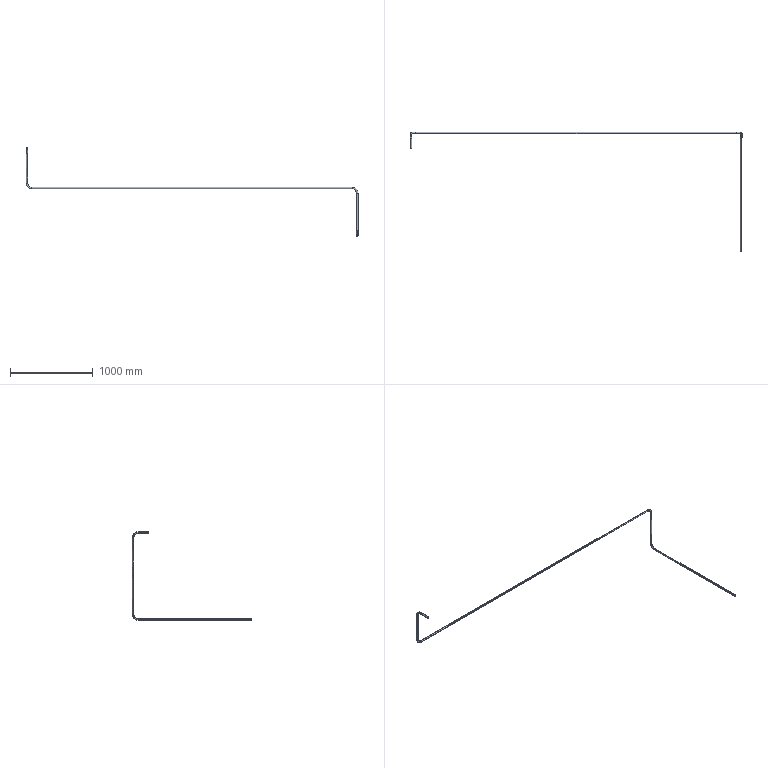Part | SolidWorks | features 3DProfileFeature 2, Sweep 1 | 1 solid | 38 faces | box 4020 x 1445 x 1070 mm | volume 1547370 mm3 | cylinder 20 | torus 16 | plane 2 | commonest cylinder face diameters 10 x10 20 x10
STEP:
#1=CARTESIAN_POINT('',(-1700.,3089.387,-104.234));
#2=VERTEX_POINT('',#1);
#3=CARTESIAN_POINT('',(-1705.,3084.387,-104.234));
#4=VERTEX_POINT('',#3);
#5=CARTESIAN_POINT('',(-1700.,3084.387,-104.234));
#6=DIRECTION('',(0.,0.,1.));
#7=DIRECTION('',(-1.,0.,0.));
#8=AXIS2_PLACEMENT_3D('',#5,#6,#7);
#9=CIRCLE('',#8,5.);
#10=EDGE_CURVE('',#2,#4,#9,.T.);
#11=ORIENTED_EDGE('',*,*,#10,.F.);
#12=CARTESIAN_POINT('',(-1700.,3024.387,-39.234));
#13=VERTEX_POINT('',#12);
#14=CARTESIAN_POINT('',(-1700.,3024.387,-104.234));
#15=DIRECTION('',(1.,0.,0.));
#16=DIRECTION('',(0.,0.,-1.));
#17=AXIS2_PLACEMENT_3D('',#14,#15,#16);
#18=CIRCLE('',#17,65.);
#19=EDGE_CURVE('',#2,#13,#18,.T.);
#20=ORIENTED_EDGE('',*,*,#19,.T.);
#21=CARTESIAN_POINT('',(-1700.,3024.387,-49.234));
#22=VERTEX_POINT('',#21);
#23=CARTESIAN_POINT('',(-1700.,3024.387,-44.234));
#24=DIRECTION('',(0.,-1.,0.));
#25=DIRECTION('',(0.,0.,-1.));
#26=AXIS2_PLACEMENT_3D('',#23,#24,#25);
#27=CIRCLE('',#26,5.);
#28=EDGE_CURVE('',#13,#22,#27,.T.);
#29=ORIENTED_EDGE('',*,*,#28,.T.);
#30=CARTESIAN_POINT('',(-1700.,3079.387,-104.234));
#31=VERTEX_POINT('',#30);
#32=CARTESIAN_POINT('',(-1700.,3024.387,-104.234));
#33=DIRECTION('',(1.,0.,0.));
#34=DIRECTION('',(0.,0.,-1.));
#35=AXIS2_PLACEMENT_3D('',#32,#33,#34);
#36=CIRCLE('',#35,55.);
#37=EDGE_CURVE('',#31,#22,#36,.T.);
#38=ORIENTED_EDGE('',*,*,#37,.F.);
#39=CARTESIAN_POINT('',(-1700.,3084.387,-104.234));
#40=DIRECTION('',(0.,0.,1.));
#41=DIRECTION('',(-1.,0.,0.));
#42=AXIS2_PLACEMENT_3D('',#39,#40,#41);
#43=CIRCLE('',#42,5.);
#44=EDGE_CURVE('',#4,#31,#43,.T.);
#45=ORIENTED_EDGE('',*,*,#44,.F.);
#46=EDGE_LOOP('',(#11,#20,#29,#38,#45));
#47=FACE_OUTER_BOUND('',#46,.T.);
#48=CARTESIAN_POINT('',(-1700.,3024.387,-104.234));
#49=DIRECTION('',(1.,0.,0.));
#50=DIRECTION('',(0.,0.,-1.));
#51=AXIS2_PLACEMENT_3D('',#48,#49,#50);
#52=TOROIDAL_SURFACE('',#51,60.,5.);
#53=ADVANCED_FACE('',(#47),#52,.F.);
#54=CARTESIAN_POINT('',(-1640.,3084.387,-526.487));
#55=VERTEX_POINT('',#54);
#56=CARTESIAN_POINT('',(-1640.,3084.387,-516.487));
#57=VERTEX_POINT('',#56);
#58=CARTESIAN_POINT('',(-1640.,3084.387,-521.487));
#59=DIRECTION('',(-1.,0.,0.));
#60=DIRECTION('',(0.,0.,-1.));
#61=AXIS2_PLACEMENT_3D('',#58,#59,#60);
#62=CIRCLE('',#61,5.);
#63=EDGE_CURVE('',#55,#57,#62,.T.);
#64=ORIENTED_EDGE('',*,*,#63,.F.);
#65=CARTESIAN_POINT('',(-1705.,3084.387,-461.487));
#66=VERTEX_POINT('',#65);
#67=CARTESIAN_POINT('',(-1640.,3084.387,-461.487));
#68=DIRECTION('',(0.,1.,0.));
#69=DIRECTION('',(0.,0.,1.));
#70=AXIS2_PLACEMENT_3D('',#67,#68,#69);
#71=CIRCLE('',#70,65.);
#72=EDGE_CURVE('',#55,#66,#71,.T.);
#73=ORIENTED_EDGE('',*,*,#72,.T.);
#74=CARTESIAN_POINT('',(-1695.,3084.387,-461.487));
#75=VERTEX_POINT('',#74);
#76=CARTESIAN_POINT('',(-1700.,3084.387,-461.487));
#77=DIRECTION('',(0.,0.,1.));
#78=DIRECTION('',(1.,0.,0.));
#79=AXIS2_PLACEMENT_3D('',#76,#77,#78);
#80=CIRCLE('',#79,5.);
#81=EDGE_CURVE('',#66,#75,#80,.T.);
#82=ORIENTED_EDGE('',*,*,#81,.T.);
#83=CARTESIAN_POINT('',(-1640.,3084.387,-461.487));
#84=DIRECTION('',(0.,1.,0.));
#85=DIRECTION('',(0.,0.,1.));
#86=AXIS2_PLACEMENT_3D('',#83,#84,#85);
#87=CIRCLE('',#86,55.);
#88=EDGE_CURVE('',#57,#75,#87,.T.);
#89=ORIENTED_EDGE('',*,*,#88,.F.);
#90=EDGE_LOOP('',(#64,#73,#82,#89));
#91=FACE_OUTER_BOUND('',#90,.T.);
#92=CARTESIAN_POINT('',(-1640.,3084.387,-461.487));
#93=DIRECTION('',(0.,1.,0.));
#94=DIRECTION('',(0.,0.,1.));
#95=AXIS2_PLACEMENT_3D('',#92,#93,#94);
#96=TOROIDAL_SURFACE('',#95,60.,5.);
#97=ADVANCED_FACE('',(#91),#96,.F.);
#98=CARTESIAN_POINT('',(2305.,3084.387,-581.487));
#99=VERTEX_POINT('',#98);
#100=CARTESIAN_POINT('',(2295.,3084.387,-581.487));
#101=VERTEX_POINT('',#100);
#102=CARTESIAN_POINT('',(2300.,3084.387,-581.487));
#103=DIRECTION('',(0.,0.,1.));
#104=DIRECTION('',(-1.,0.,0.));
#105=AXIS2_PLACEMENT_3D('',#102,#103,#104);
#106=CIRCLE('',#105,5.);
#107=EDGE_CURVE('',#99,#101,#106,.T.);
#108=ORIENTED_EDGE('',*,*,#107,.F.);
#109=CARTESIAN_POINT('',(2240.,3084.387,-516.487));
#110=VERTEX_POINT('',#109);
#111=CARTESIAN_POINT('',(2240.,3084.387,-581.487));
#112=DIRECTION('',(0.,-1.,0.));
#113=DIRECTION('',(0.,0.,-1.));
#114=AXIS2_PLACEMENT_3D('',#111,#112,#113);
#115=CIRCLE('',#114,65.);
#116=EDGE_CURVE('',#99,#110,#115,.T.);
#117=ORIENTED_EDGE('',*,*,#116,.T.);
#118=CARTESIAN_POINT('',(2240.,3084.387,-526.487));
#119=VERTEX_POINT('',#118);
#120=CARTESIAN_POINT('',(2240.,3084.387,-521.487));
#121=DIRECTION('',(-1.,0.,0.));
#122=DIRECTION('',(0.,0.,1.));
#123=AXIS2_PLACEMENT_3D('',#120,#121,#122);
#124=CIRCLE('',#123,5.);
#125=EDGE_CURVE('',#110,#119,#124,.T.);
#126=ORIENTED_EDGE('',*,*,#125,.T.);
#127=CARTESIAN_POINT('',(2240.,3084.387,-581.487));
#128=DIRECTION('',(0.,-1.,0.));
#129=DIRECTION('',(0.,0.,-1.));
#130=AXIS2_PLACEMENT_3D('',#127,#128,#129);
#131=CIRCLE('',#130,55.);
#132=EDGE_CURVE('',#101,#119,#131,.T.);
#133=ORIENTED_EDGE('',*,*,#132,.F.);
#134=EDGE_LOOP('',(#108,#117,#126,#133));
#135=FACE_OUTER_BOUND('',#134,.T.);
#136=CARTESIAN_POINT('',(2240.,3084.387,-581.487));
#137=DIRECTION('',(0.,-1.,0.));
#138=DIRECTION('',(0.,0.,-1.));
#139=AXIS2_PLACEMENT_3D('',#136,#137,#138);
#140=TOROIDAL_SURFACE('',#139,60.,5.);
#141=ADVANCED_FACE('',(#135),#140,.F.);
#142=CARTESIAN_POINT('',(2300.,3024.387,-1099.234));
#143=VERTEX_POINT('',#142);
#144=CARTESIAN_POINT('',(2300.,3024.387,-1089.234));
#145=VERTEX_POINT('',#144);
#146=CARTESIAN_POINT('',(2300.,3024.387,-1094.234));
#147=DIRECTION('',(0.,1.,0.));
#148=DIRECTION('',(0.,0.,-1.));
#149=AXIS2_PLACEMENT_3D('',#146,#147,#148);
#150=CIRCLE('',#149,5.);
#151=EDGE_CURVE('',#143,#145,#150,.T.);
#152=ORIENTED_EDGE('',*,*,#151,.F.);
#153=CARTESIAN_POINT('',(2300.,3089.387,-1034.234));
#154=VERTEX_POINT('',#153);
#155=CARTESIAN_POINT('',(2300.,3024.387,-1034.234));
#156=DIRECTION('',(1.,0.,0.));
#157=DIRECTION('',(0.,0.,-1.));
#158=AXIS2_PLACEMENT_3D('',#155,#156,#157);
#159=CIRCLE('',#158,65.);
#160=EDGE_CURVE('',#143,#154,#159,.T.);
#161=ORIENTED_EDGE('',*,*,#160,.T.);
#162=CARTESIAN_POINT('',(2295.,3084.387,-1034.234));
#163=VERTEX_POINT('',#162);
#164=CARTESIAN_POINT('',(2300.,3084.387,-1034.234));
#165=DIRECTION('',(0.,0.,1.));
#166=DIRECTION('',(1.,0.,0.));
#167=AXIS2_PLACEMENT_3D('',#164,#165,#166);
#168=CIRCLE('',#167,5.);
#169=EDGE_CURVE('',#154,#163,#168,.T.);
#170=ORIENTED_EDGE('',*,*,#169,.T.);
#171=CARTESIAN_POINT('',(2300.,3079.387,-1034.234));
#172=VERTEX_POINT('',#171);
#173=CARTESIAN_POINT('',(2300.,3084.387,-1034.234));
#174=DIRECTION('',(0.,0.,1.));
#175=DIRECTION('',(1.,0.,0.));
#176=AXIS2_PLACEMENT_3D('',#173,#174,#175);
#177=CIRCLE('',#176,5.);
#178=EDGE_CURVE('',#163,#172,#177,.T.);
#179=ORIENTED_EDGE('',*,*,#178,.T.);
#180=CARTESIAN_POINT('',(2300.,3024.387,-1034.234));
#181=DIRECTION('',(1.,0.,0.));
#182=DIRECTION('',(0.,0.,-1.));
#183=AXIS2_PLACEMENT_3D('',#180,#181,#182);
#184=CIRCLE('',#183,55.);
#185=EDGE_CURVE('',#145,#172,#184,.T.);
#186=ORIENTED_EDGE('',*,*,#185,.F.);
#187=EDGE_LOOP('',(#152,#161,#170,#179,#186));
#188=FACE_OUTER_BOUND('',#187,.T.);
#189=CARTESIAN_POINT('',(2300.,3024.387,-1034.234));
#190=DIRECTION('',(1.,0.,0.));
#191=DIRECTION('',(0.,0.,-1.));
#192=AXIS2_PLACEMENT_3D('',#189,#190,#191);
#193=TOROIDAL_SURFACE('',#192,60.,5.);
#194=ADVANCED_FACE('',(#188),#193,.F.);
#195=CARTESIAN_POINT('',(-1690.,3084.387,-104.234));
#196=VERTEX_POINT('',#195);
#197=CARTESIAN_POINT('',(-1700.,3094.387,-104.234));
#198=VERTEX_POINT('',#197);
#199=CARTESIAN_POINT('',(-1700.,3084.387,-104.234));
#200=DIRECTION('',(0.,0.,1.));
#201=DIRECTION('',(0.,-1.,0.));
#202=AXIS2_PLACEMENT_3D('',#199,#200,#201);
#203=CIRCLE('',#202,10.);
#204=EDGE_CURVE('',#196,#198,#203,.T.);
#205=ORIENTED_EDGE('',*,*,#204,.T.);
#206=CARTESIAN_POINT('',(-1700.,3024.387,-34.234));
#207=VERTEX_POINT('',#206);
#208=CARTESIAN_POINT('',(-1700.,3024.387,-104.234));
#209=DIRECTION('',(1.,0.,0.));
#210=DIRECTION('',(0.,0.,-1.));
#211=AXIS2_PLACEMENT_3D('',#208,#209,#210);
#212=CIRCLE('',#211,70.);
#213=EDGE_CURVE('',#198,#207,#212,.T.);
#214=ORIENTED_EDGE('',*,*,#213,.T.);
#215=CARTESIAN_POINT('',(-1700.,3024.387,-54.234));
#216=VERTEX_POINT('',#215);
#217=CARTESIAN_POINT('',(-1700.,3024.387,-44.234));
#218=DIRECTION('',(0.,-1.,0.));
#219=DIRECTION('',(0.,0.,-1.));
#220=AXIS2_PLACEMENT_3D('',#217,#218,#219);
#221=CIRCLE('',#220,10.);
#222=EDGE_CURVE('',#216,#207,#221,.T.);
#223=ORIENTED_EDGE('',*,*,#222,.F.);
#224=CARTESIAN_POINT('',(-1700.,3074.387,-104.234));
#225=VERTEX_POINT('',#224);
#226=CARTESIAN_POINT('',(-1700.,3024.387,-104.234));
#227=DIRECTION('',(1.,0.,0.));
#228=DIRECTION('',(0.,0.,-1.));
#229=AXIS2_PLACEMENT_3D('',#226,#227,#228);
#230=CIRCLE('',#229,50.);
#231=EDGE_CURVE('',#225,#216,#230,.T.);
#232=ORIENTED_EDGE('',*,*,#231,.F.);
#233=CARTESIAN_POINT('',(-1700.,3084.387,-104.234));
#234=DIRECTION('',(0.,0.,1.));
#235=DIRECTION('',(0.,-1.,0.));
#236=AXIS2_PLACEMENT_3D('',#233,#234,#235);
#237=CIRCLE('',#236,10.);
#238=EDGE_CURVE('',#225,#196,#237,.T.);
#239=ORIENTED_EDGE('',*,*,#238,.T.);
#240=EDGE_LOOP('',(#205,#214,#223,#232,#239));
#241=FACE_OUTER_BOUND('',#240,.T.);
#242=CARTESIAN_POINT('',(-1700.,3024.387,-104.234));
#243=DIRECTION('',(1.,0.,0.));
#244=DIRECTION('',(0.,0.,-1.));
#245=AXIS2_PLACEMENT_3D('',#242,#243,#244);
#246=TOROIDAL_SURFACE('',#245,60.,10.);
#247=ADVANCED_FACE('',(#241),#246,.T.);
#248=CARTESIAN_POINT('',(-1640.,3084.387,-511.487));
#249=VERTEX_POINT('',#248);
#250=CARTESIAN_POINT('',(-1640.,3084.387,-531.487));
#251=VERTEX_POINT('',#250);
#252=CARTESIAN_POINT('',(-1640.,3084.387,-521.487));
#253=DIRECTION('',(-1.,0.,0.));
#254=DIRECTION('',(0.,-1.,0.));
#255=AXIS2_PLACEMENT_3D('',#252,#253,#254);
#256=CIRCLE('',#255,10.);
#257=EDGE_CURVE('',#249,#251,#256,.T.);
#258=ORIENTED_EDGE('',*,*,#257,.T.);
#259=CARTESIAN_POINT('',(-1710.,3084.387,-461.487));
#260=VERTEX_POINT('',#259);
#261=CARTESIAN_POINT('',(-1640.,3084.387,-461.487));
#262=DIRECTION('',(0.,1.,0.));
#263=DIRECTION('',(0.,0.,1.));
#264=AXIS2_PLACEMENT_3D('',#261,#262,#263);
#265=CIRCLE('',#264,70.);
#266=EDGE_CURVE('',#251,#260,#265,.T.);
#267=ORIENTED_EDGE('',*,*,#266,.T.);
#268=CARTESIAN_POINT('',(-1690.,3084.387,-461.487));
#269=VERTEX_POINT('',#268);
#270=CARTESIAN_POINT('',(-1700.,3084.387,-461.487));
#271=DIRECTION('',(0.,0.,1.));
#272=DIRECTION('',(0.,-1.,0.));
#273=AXIS2_PLACEMENT_3D('',#270,#271,#272);
#274=CIRCLE('',#273,10.);
#275=EDGE_CURVE('',#269,#260,#274,.T.);
#276=ORIENTED_EDGE('',*,*,#275,.F.);
#277=CARTESIAN_POINT('',(-1640.,3084.387,-461.487));
#278=DIRECTION('',(0.,1.,0.));
#279=DIRECTION('',(0.,0.,1.));
#280=AXIS2_PLACEMENT_3D('',#277,#278,#279);
#281=CIRCLE('',#280,50.);
#282=EDGE_CURVE('',#249,#269,#281,.T.);
#283=ORIENTED_EDGE('',*,*,#282,.F.);
#284=EDGE_LOOP('',(#258,#267,#276,#283));
#285=FACE_OUTER_BOUND('',#284,.T.);
#286=CARTESIAN_POINT('',(-1640.,3084.387,-461.487));
#287=DIRECTION('',(0.,1.,0.));
#288=DIRECTION('',(0.,0.,1.));
#289=AXIS2_PLACEMENT_3D('',#286,#287,#288);
#290=TOROIDAL_SURFACE('',#289,60.,10.);
#291=ADVANCED_FACE('',(#285),#290,.T.);
#292=CARTESIAN_POINT('',(2290.,3084.387,-581.487));
#293=VERTEX_POINT('',#292);
#294=CARTESIAN_POINT('',(2310.,3084.387,-581.487));
#295=VERTEX_POINT('',#294);
#296=CARTESIAN_POINT('',(2300.,3084.387,-581.487));
#297=DIRECTION('',(0.,0.,1.));
#298=DIRECTION('',(0.,-1.,0.));
#299=AXIS2_PLACEMENT_3D('',#296,#297,#298);
#300=CIRCLE('',#299,10.);
#301=EDGE_CURVE('',#293,#295,#300,.T.);
#302=ORIENTED_EDGE('',*,*,#301,.T.);
#303=CARTESIAN_POINT('',(2240.,3084.387,-511.487));
#304=VERTEX_POINT('',#303);
#305=CARTESIAN_POINT('',(2240.,3084.387,-581.487));
#306=DIRECTION('',(0.,-1.,0.));
#307=DIRECTION('',(0.,0.,-1.));
#308=AXIS2_PLACEMENT_3D('',#305,#306,#307);
#309=CIRCLE('',#308,70.);
#310=EDGE_CURVE('',#295,#304,#309,.T.);
#311=ORIENTED_EDGE('',*,*,#310,.T.);
#312=CARTESIAN_POINT('',(2240.,3084.387,-531.487));
#313=VERTEX_POINT('',#312);
#314=CARTESIAN_POINT('',(2240.,3084.387,-521.487));
#315=DIRECTION('',(-1.,0.,0.));
#316=DIRECTION('',(0.,-1.,0.));
#317=AXIS2_PLACEMENT_3D('',#314,#315,#316);
#318=CIRCLE('',#317,10.);
#319=EDGE_CURVE('',#313,#304,#318,.T.);
#320=ORIENTED_EDGE('',*,*,#319,.F.);
#321=CARTESIAN_POINT('',(2240.,3084.387,-581.487));
#322=DIRECTION('',(0.,-1.,0.));
#323=DIRECTION('',(0.,0.,-1.));
#324=AXIS2_PLACEMENT_3D('',#321,#322,#323);
#325=CIRCLE('',#324,50.);
#326=EDGE_CURVE('',#293,#313,#325,.T.);
#327=ORIENTED_EDGE('',*,*,#326,.F.);
#328=EDGE_LOOP('',(#302,#311,#320,#327));
#329=FACE_OUTER_BOUND('',#328,.T.);
#330=CARTESIAN_POINT('',(2240.,3084.387,-581.487));
#331=DIRECTION('',(0.,-1.,0.));
#332=DIRECTION('',(0.,0.,-1.));
#333=AXIS2_PLACEMENT_3D('',#330,#331,#332);
#334=TOROIDAL_SURFACE('',#333,60.,10.);
#335=ADVANCED_FACE('',(#329),#334,.T.);
#336=CARTESIAN_POINT('',(2300.,3024.387,-1084.234));
#337=VERTEX_POINT('',#336);
#338=CARTESIAN_POINT('',(2300.,3024.387,-1104.234));
#339=VERTEX_POINT('',#338);
#340=CARTESIAN_POINT('',(2300.,3024.387,-1094.234));
#341=DIRECTION('',(0.,1.,0.));
#342=DIRECTION('',(0.,0.,1.));
#343=AXIS2_PLACEMENT_3D('',#340,#341,#342);
#344=CIRCLE('',#343,10.);
#345=EDGE_CURVE('',#337,#339,#344,.T.);
#346=ORIENTED_EDGE('',*,*,#345,.T.);
#347=CARTESIAN_POINT('',(2300.,3094.387,-1034.234));
#348=VERTEX_POINT('',#347);
#349=CARTESIAN_POINT('',(2300.,3024.387,-1034.234));
#350=DIRECTION('',(1.,0.,0.));
#351=DIRECTION('',(0.,0.,-1.));
#352=AXIS2_PLACEMENT_3D('',#349,#350,#351);
#353=CIRCLE('',#352,70.);
#354=EDGE_CURVE('',#339,#348,#353,.T.);
#355=ORIENTED_EDGE('',*,*,#354,.T.);
#356=CARTESIAN_POINT('',(2310.,3084.387,-1034.234));
#357=VERTEX_POINT('',#356);
#358=CARTESIAN_POINT('',(2300.,3084.387,-1034.234));
#359=DIRECTION('',(0.,0.,1.));
#360=DIRECTION('',(0.,-1.,0.));
#361=AXIS2_PLACEMENT_3D('',#358,#359,#360);
#362=CIRCLE('',#361,10.);
#363=EDGE_CURVE('',#357,#348,#362,.T.);
#364=ORIENTED_EDGE('',*,*,#363,.F.);
#365=CARTESIAN_POINT('',(2300.,3074.387,-1034.234));
#366=VERTEX_POINT('',#365);
#367=CARTESIAN_POINT('',(2300.,3084.387,-1034.234));
#368=DIRECTION('',(0.,0.,1.));
#369=DIRECTION('',(0.,-1.,0.));
#370=AXIS2_PLACEMENT_3D('',#367,#368,#369);
#371=CIRCLE('',#370,10.);
#372=EDGE_CURVE('',#366,#357,#371,.T.);
#373=ORIENTED_EDGE('',*,*,#372,.F.);
#374=CARTESIAN_POINT('',(2300.,3024.387,-1034.234));
#375=DIRECTION('',(1.,0.,0.));
#376=DIRECTION('',(0.,0.,-1.));
#377=AXIS2_PLACEMENT_3D('',#374,#375,#376);
#378=CIRCLE('',#377,50.);
#379=EDGE_CURVE('',#337,#366,#378,.T.);
#380=ORIENTED_EDGE('',*,*,#379,.F.);
#381=EDGE_LOOP('',(#346,#355,#364,#373,#380));
#382=FACE_OUTER_BOUND('',#381,.T.);
#383=CARTESIAN_POINT('',(2300.,3024.387,-1034.234));
#384=DIRECTION('',(1.,0.,0.));
#385=DIRECTION('',(0.,0.,-1.));
#386=AXIS2_PLACEMENT_3D('',#383,#384,#385);
#387=TOROIDAL_SURFACE('',#386,60.,10.);
#388=ADVANCED_FACE('',(#382),#387,.T.);
#389=ORIENTED_EDGE('',*,*,#28,.F.);
#390=CARTESIAN_POINT('',(-1700.,2899.052,-39.234));
#391=VERTEX_POINT('',#390);
#392=CARTESIAN_POINT('',(-1700.,3024.387,-39.234));
#393=DIRECTION('',(0.,-1.,0.));
#394=VECTOR('',#393,1000.);
#395=LINE('',#392,#394);
#396=EDGE_CURVE('',#13,#391,#395,.T.);
#397=ORIENTED_EDGE('',*,*,#396,.T.);
#398=CARTESIAN_POINT('',(-1700.,2899.052,-49.234));
#399=VERTEX_POINT('',#398);
#400=CARTESIAN_POINT('',(-1700.,2899.052,-44.234));
#401=DIRECTION('',(0.,-1.,0.));
#402=DIRECTION('',(0.,0.,-1.));
#403=AXIS2_PLACEMENT_3D('',#400,#401,#402);
#404=CIRCLE('',#403,5.);
#405=EDGE_CURVE('',#391,#399,#404,.T.);
#406=ORIENTED_EDGE('',*,*,#405,.T.);
#407=CARTESIAN_POINT('',(-1700.,3024.387,-49.234));
#408=DIRECTION('',(0.,-1.,0.));
#409=VECTOR('',#408,1000.);
#410=LINE('',#407,#409);
#411=EDGE_CURVE('',#22,#399,#410,.T.);
#412=ORIENTED_EDGE('',*,*,#411,.F.);
#413=EDGE_LOOP('',(#389,#397,#406,#412));
#414=FACE_OUTER_BOUND('',#413,.T.);
#415=CARTESIAN_POINT('',(-1700.,3024.387,-44.234));
#416=DIRECTION('',(0.,-1.,0.));
#417=DIRECTION('',(0.,0.,-1.));
#418=AXIS2_PLACEMENT_3D('',#415,#416,#417);
#419=CYLINDRICAL_SURFACE('',#418,5.);
#420=ADVANCED_FACE('',(#414),#419,.F.);
#421=ORIENTED_EDGE('',*,*,#81,.F.);
#422=CARTESIAN_POINT('',(-1705.,3084.387,-461.487));
#423=DIRECTION('',(0.,0.,1.));
#424=VECTOR('',#423,1000.);
#425=LINE('',#422,#424);
#426=EDGE_CURVE('',#66,#4,#425,.T.);
#427=ORIENTED_EDGE('',*,*,#426,.T.);
#428=ORIENTED_EDGE('',*,*,#44,.T.);
#429=CARTESIAN_POINT('',(-1695.,3084.387,-104.234));
#430=VERTEX_POINT('',#429);
#431=CARTESIAN_POINT('',(-1700.,3084.387,-104.234));
#432=DIRECTION('',(0.,0.,1.));
#433=DIRECTION('',(-1.,0.,0.));
#434=AXIS2_PLACEMENT_3D('',#431,#432,#433);
#435=CIRCLE('',#434,5.);
#436=EDGE_CURVE('',#31,#430,#435,.T.);
#437=ORIENTED_EDGE('',*,*,#436,.T.);
#438=CARTESIAN_POINT('',(-1695.,3084.387,-461.487));
#439=DIRECTION('',(0.,0.,1.));
#440=VECTOR('',#439,1000.);
#441=LINE('',#438,#440);
#442=EDGE_CURVE('',#75,#430,#441,.T.);
#443=ORIENTED_EDGE('',*,*,#442,.F.);
#444=EDGE_LOOP('',(#421,#427,#428,#437,#443));
#445=FACE_OUTER_BOUND('',#444,.T.);
#446=CARTESIAN_POINT('',(-1700.,3084.387,-461.487));
#447=DIRECTION('',(0.,0.,1.));
#448=DIRECTION('',(1.,0.,0.));
#449=AXIS2_PLACEMENT_3D('',#446,#447,#448);
#450=CYLINDRICAL_SURFACE('',#449,5.);
#451=ADVANCED_FACE('',(#445),#450,.F.);
#452=CARTESIAN_POINT('',(2240.,3084.387,-521.487));
#453=DIRECTION('',(-1.,0.,0.));
#454=DIRECTION('',(0.,0.,1.));
#455=AXIS2_PLACEMENT_3D('',#452,#453,#454);
#456=CIRCLE('',#455,5.);
#457=EDGE_CURVE('',#119,#110,#456,.T.);
#458=ORIENTED_EDGE('',*,*,#457,.F.);
#459=CARTESIAN_POINT('',(2240.,3084.387,-526.487));
#460=DIRECTION('',(-1.,0.,0.));
#461=VECTOR('',#460,1000.);
#462=LINE('',#459,#461);
#463=EDGE_CURVE('',#119,#55,#462,.T.);
#464=ORIENTED_EDGE('',*,*,#463,.T.);
#465=ORIENTED_EDGE('',*,*,#63,.T.);
#466=CARTESIAN_POINT('',(2240.,3084.387,-516.487));
#467=DIRECTION('',(-1.,0.,0.));
#468=VECTOR('',#467,1000.);
#469=LINE('',#466,#468);
#470=EDGE_CURVE('',#110,#57,#469,.T.);
#471=ORIENTED_EDGE('',*,*,#470,.F.);
#472=EDGE_LOOP('',(#458,#464,#465,#471));
#473=FACE_OUTER_BOUND('',#472,.T.);
#474=CARTESIAN_POINT('',(2240.,3084.387,-521.487));
#475=DIRECTION('',(-1.,0.,0.));
#476=DIRECTION('',(0.,0.,1.));
#477=AXIS2_PLACEMENT_3D('',#474,#475,#476);
#478=CYLINDRICAL_SURFACE('',#477,5.);
#479=ADVANCED_FACE('',(#473),#478,.F.);
#480=ORIENTED_EDGE('',*,*,#178,.F.);
#481=CARTESIAN_POINT('',(2295.,3084.387,-1034.234));
#482=DIRECTION('',(0.,0.,1.));
#483=VECTOR('',#482,1000.);
#484=LINE('',#481,#483);
#485=EDGE_CURVE('',#163,#101,#484,.T.);
#486=ORIENTED_EDGE('',*,*,#485,.T.);
#487=CARTESIAN_POINT('',(2300.,3084.387,-581.487));
#488=DIRECTION('',(0.,0.,1.));
#489=DIRECTION('',(-1.,0.,0.));
#490=AXIS2_PLACEMENT_3D('',#487,#488,#489);
#491=CIRCLE('',#490,5.);
#492=EDGE_CURVE('',#101,#99,#491,.T.);
#493=ORIENTED_EDGE('',*,*,#492,.T.);
#494=CARTESIAN_POINT('',(2305.,3084.387,-1034.234));
#495=VERTEX_POINT('',#494);
#496=CARTESIAN_POINT('',(2305.,3084.387,-1034.234));
#497=DIRECTION('',(0.,0.,1.));
#498=VECTOR('',#497,1000.);
#499=LINE('',#496,#498);
#500=EDGE_CURVE('',#495,#99,#499,.T.);
#501=ORIENTED_EDGE('',*,*,#500,.F.);
#502=CARTESIAN_POINT('',(2300.,3084.387,-1034.234));
#503=DIRECTION('',(0.,0.,1.));
#504=DIRECTION('',(1.,0.,0.));
#505=AXIS2_PLACEMENT_3D('',#502,#503,#504);
#506=CIRCLE('',#505,5.);
#507=EDGE_CURVE('',#172,#495,#506,.T.);
#508=ORIENTED_EDGE('',*,*,#507,.F.);
#509=EDGE_LOOP('',(#480,#486,#493,#501,#508));
#510=FACE_OUTER_BOUND('',#509,.T.);
#511=CARTESIAN_POINT('',(2300.,3084.387,-1034.234));
#512=DIRECTION('',(0.,0.,1.));
#513=DIRECTION('',(1.,0.,0.));
#514=AXIS2_PLACEMENT_3D('',#511,#512,#513);
#515=CYLINDRICAL_SURFACE('',#514,5.);
#516=ADVANCED_FACE('',(#510),#515,.F.);
#517=CARTESIAN_POINT('',(2300.,1649.47,-1099.234));
#518=VERTEX_POINT('',#517);
#519=CARTESIAN_POINT('',(2300.,1649.47,-1089.234));
#520=VERTEX_POINT('',#519);
#521=CARTESIAN_POINT('',(2300.,1649.47,-1094.234));
#522=DIRECTION('',(0.,1.,0.));
#523=DIRECTION('',(0.,0.,1.));
#524=AXIS2_PLACEMENT_3D('',#521,#522,#523);
#525=CIRCLE('',#524,5.);
#526=EDGE_CURVE('',#518,#520,#525,.T.);
#527=ORIENTED_EDGE('',*,*,#526,.F.);
#528=CARTESIAN_POINT('',(2300.,1649.47,-1099.234));
#529=DIRECTION('',(0.,1.,0.));
#530=VECTOR('',#529,1000.);
#531=LINE('',#528,#530);
#532=EDGE_CURVE('',#518,#143,#531,.T.);
#533=ORIENTED_EDGE('',*,*,#532,.T.);
#534=ORIENTED_EDGE('',*,*,#151,.T.);
#535=CARTESIAN_POINT('',(2300.,1649.47,-1089.234));
#536=DIRECTION('',(0.,1.,0.));
#537=VECTOR('',#536,1000.);
#538=LINE('',#535,#537);
#539=EDGE_CURVE('',#520,#145,#538,.T.);
#540=ORIENTED_EDGE('',*,*,#539,.F.);
#541=EDGE_LOOP('',(#527,#533,#534,#540));
#542=FACE_OUTER_BOUND('',#541,.T.);
#543=CARTESIAN_POINT('',(2300.,1649.47,-1094.234));
#544=DIRECTION('',(0.,1.,0.));
#545=DIRECTION('',(0.,0.,1.));
#546=AXIS2_PLACEMENT_3D('',#543,#544,#545);
#547=CYLINDRICAL_SURFACE('',#546,5.);
#548=ADVANCED_FACE('',(#542),#547,.F.);
#549=ORIENTED_EDGE('',*,*,#222,.T.);
#550=CARTESIAN_POINT('',(-1700.,2899.052,-34.234));
#551=VERTEX_POINT('',#550);
#552=CARTESIAN_POINT('',(-1700.,3024.387,-34.234));
#553=DIRECTION('',(0.,-1.,0.));
#554=VECTOR('',#553,1000.);
#555=LINE('',#552,#554);
#556=EDGE_CURVE('',#207,#551,#555,.T.);
#557=ORIENTED_EDGE('',*,*,#556,.T.);
#558=CARTESIAN_POINT('',(-1700.,2899.052,-54.234));
#559=VERTEX_POINT('',#558);
#560=CARTESIAN_POINT('',(-1700.,2899.052,-44.234));
#561=DIRECTION('',(0.,-1.,0.));
#562=DIRECTION('',(0.,0.,-1.));
#563=AXIS2_PLACEMENT_3D('',#560,#561,#562);
#564=CIRCLE('',#563,10.);
#565=EDGE_CURVE('',#559,#551,#564,.T.);
#566=ORIENTED_EDGE('',*,*,#565,.F.);
#567=CARTESIAN_POINT('',(-1700.,3024.387,-54.234));
#568=DIRECTION('',(0.,-1.,0.));
#569=VECTOR('',#568,1000.);
#570=LINE('',#567,#569);
#571=EDGE_CURVE('',#216,#559,#570,.T.);
#572=ORIENTED_EDGE('',*,*,#571,.F.);
#573=EDGE_LOOP('',(#549,#557,#566,#572));
#574=FACE_OUTER_BOUND('',#573,.T.);
#575=CARTESIAN_POINT('',(-1700.,3024.387,-44.234));
#576=DIRECTION('',(0.,-1.,0.));
#577=DIRECTION('',(0.,0.,-1.));
#578=AXIS2_PLACEMENT_3D('',#575,#576,#577);
#579=CYLINDRICAL_SURFACE('',#578,10.);
#580=ADVANCED_FACE('',(#574),#579,.T.);
#581=ORIENTED_EDGE('',*,*,#275,.T.);
#582=CARTESIAN_POINT('',(-1710.,3084.387,-104.234));
#583=VERTEX_POINT('',#582);
#584=CARTESIAN_POINT('',(-1710.,3084.387,-461.487));
#585=DIRECTION('',(0.,0.,1.));
#586=VECTOR('',#585,1000.);
#587=LINE('',#584,#586);
#588=EDGE_CURVE('',#260,#583,#587,.T.);
#589=ORIENTED_EDGE('',*,*,#588,.T.);
#590=CARTESIAN_POINT('',(-1700.,3084.387,-104.234));
#591=DIRECTION('',(0.,0.,1.));
#592=DIRECTION('',(0.,-1.,0.));
#593=AXIS2_PLACEMENT_3D('',#590,#591,#592);
#594=CIRCLE('',#593,10.);
#595=EDGE_CURVE('',#198,#583,#594,.T.);
#596=ORIENTED_EDGE('',*,*,#595,.F.);
#597=ORIENTED_EDGE('',*,*,#204,.F.);
#598=CARTESIAN_POINT('',(-1690.,3084.387,-461.487));
#599=DIRECTION('',(0.,0.,1.));
#600=VECTOR('',#599,1000.);
#601=LINE('',#598,#600);
#602=EDGE_CURVE('',#269,#196,#601,.T.);
#603=ORIENTED_EDGE('',*,*,#602,.F.);
#604=EDGE_LOOP('',(#581,#589,#596,#597,#603));
#605=FACE_OUTER_BOUND('',#604,.T.);
#606=CARTESIAN_POINT('',(-1700.,3084.387,-461.487));
#607=DIRECTION('',(0.,0.,1.));
#608=DIRECTION('',(1.,0.,0.));
#609=AXIS2_PLACEMENT_3D('',#606,#607,#608);
#610=CYLINDRICAL_SURFACE('',#609,10.);
#611=ADVANCED_FACE('',(#605),#610,.T.);
#612=CARTESIAN_POINT('',(2240.,3084.387,-521.487));
#613=DIRECTION('',(-1.,0.,0.));
#614=DIRECTION('',(0.,-1.,0.));
#615=AXIS2_PLACEMENT_3D('',#612,#613,#614);
#616=CIRCLE('',#615,10.);
#617=EDGE_CURVE('',#304,#313,#616,.T.);
#618=ORIENTED_EDGE('',*,*,#617,.T.);
#619=CARTESIAN_POINT('',(2240.,3084.387,-531.487));
#620=DIRECTION('',(-1.,0.,0.));
#621=VECTOR('',#620,1000.);
#622=LINE('',#619,#621);
#623=EDGE_CURVE('',#313,#251,#622,.T.);
#624=ORIENTED_EDGE('',*,*,#623,.T.);
#625=ORIENTED_EDGE('',*,*,#257,.F.);
#626=CARTESIAN_POINT('',(2240.,3084.387,-511.487));
#627=DIRECTION('',(-1.,0.,0.));
#628=VECTOR('',#627,1000.);
#629=LINE('',#626,#628);
#630=EDGE_CURVE('',#304,#249,#629,.T.);
#631=ORIENTED_EDGE('',*,*,#630,.F.);
#632=EDGE_LOOP('',(#618,#624,#625,#631));
#633=FACE_OUTER_BOUND('',#632,.T.);
#634=CARTESIAN_POINT('',(2240.,3084.387,-521.487));
#635=DIRECTION('',(-1.,0.,0.));
#636=DIRECTION('',(0.,0.,1.));
#637=AXIS2_PLACEMENT_3D('',#634,#635,#636);
#638=CYLINDRICAL_SURFACE('',#637,10.);
#639=ADVANCED_FACE('',(#633),#638,.T.);
#640=ORIENTED_EDGE('',*,*,#363,.T.);
#641=CARTESIAN_POINT('',(2290.,3084.387,-1034.234));
#642=VERTEX_POINT('',#641);
#643=CARTESIAN_POINT('',(2300.,3084.387,-1034.234));
#644=DIRECTION('',(0.,0.,1.));
#645=DIRECTION('',(0.,-1.,0.));
#646=AXIS2_PLACEMENT_3D('',#643,#644,#645);
#647=CIRCLE('',#646,10.);
#648=EDGE_CURVE('',#348,#642,#647,.T.);
#649=ORIENTED_EDGE('',*,*,#648,.T.);
#650=CARTESIAN_POINT('',(2290.,3084.387,-1034.234));
#651=DIRECTION('',(0.,0.,1.));
#652=VECTOR('',#651,1000.);
#653=LINE('',#650,#652);
#654=EDGE_CURVE('',#642,#293,#653,.T.);
#655=ORIENTED_EDGE('',*,*,#654,.T.);
#656=CARTESIAN_POINT('',(2300.,3084.387,-581.487));
#657=DIRECTION('',(0.,0.,1.));
#658=DIRECTION('',(0.,-1.,0.));
#659=AXIS2_PLACEMENT_3D('',#656,#657,#658);
#660=CIRCLE('',#659,10.);
#661=EDGE_CURVE('',#295,#293,#660,.T.);
#662=ORIENTED_EDGE('',*,*,#661,.F.);
#663=CARTESIAN_POINT('',(2310.,3084.387,-1034.234));
#664=DIRECTION('',(0.,0.,1.));
#665=VECTOR('',#664,1000.);
#666=LINE('',#663,#665);
#667=EDGE_CURVE('',#357,#295,#666,.T.);
#668=ORIENTED_EDGE('',*,*,#667,.F.);
#669=EDGE_LOOP('',(#640,#649,#655,#662,#668));
#670=FACE_OUTER_BOUND('',#669,.T.);
#671=CARTESIAN_POINT('',(2300.,3084.387,-1034.234));
#672=DIRECTION('',(0.,0.,1.));
#673=DIRECTION('',(1.,0.,0.));
#674=AXIS2_PLACEMENT_3D('',#671,#672,#673);
#675=CYLINDRICAL_SURFACE('',#674,10.);
#676=ADVANCED_FACE('',(#670),#675,.T.);
#677=CARTESIAN_POINT('',(2300.,1649.47,-1084.234));
#678=VERTEX_POINT('',#677);
#679=CARTESIAN_POINT('',(2300.,1649.47,-1104.234));
#680=VERTEX_POINT('',#679);
#681=CARTESIAN_POINT('',(2300.,1649.47,-1094.234));
#682=DIRECTION('',(0.,1.,0.));
#683=DIRECTION('',(0.,0.,1.));
#684=AXIS2_PLACEMENT_3D('',#681,#682,#683);
#685=CIRCLE('',#684,10.);
#686=EDGE_CURVE('',#678,#680,#685,.T.);
#687=ORIENTED_EDGE('',*,*,#686,.T.);
#688=CARTESIAN_POINT('',(2300.,1649.47,-1104.234));
#689=DIRECTION('',(0.,1.,0.));
#690=VECTOR('',#689,1000.);
#691=LINE('',#688,#690);
#692=EDGE_CURVE('',#680,#339,#691,.T.);
#693=ORIENTED_EDGE('',*,*,#692,.T.);
#694=ORIENTED_EDGE('',*,*,#345,.F.);
#695=CARTESIAN_POINT('',(2300.,1649.47,-1084.234));
#696=DIRECTION('',(0.,1.,0.));
#697=VECTOR('',#696,1000.);
#698=LINE('',#695,#697);
#699=EDGE_CURVE('',#678,#337,#698,.T.);
#700=ORIENTED_EDGE('',*,*,#699,.F.);
#701=EDGE_LOOP('',(#687,#693,#694,#700));
#702=FACE_OUTER_BOUND('',#701,.T.);
#703=CARTESIAN_POINT('',(2300.,1649.47,-1094.234));
#704=DIRECTION('',(0.,1.,0.));
#705=DIRECTION('',(0.,0.,1.));
#706=AXIS2_PLACEMENT_3D('',#703,#704,#705);
#707=CYLINDRICAL_SURFACE('',#706,10.);
#708=ADVANCED_FACE('',(#702),#707,.T.);
#709=ORIENTED_EDGE('',*,*,#556,.F.);
#710=CARTESIAN_POINT('',(-1700.,3024.387,-44.234));
#711=DIRECTION('',(0.,-1.,0.));
#712=DIRECTION('',(0.,0.,-1.));
#713=AXIS2_PLACEMENT_3D('',#710,#711,#712);
#714=CIRCLE('',#713,10.);
#715=EDGE_CURVE('',#207,#216,#714,.T.);
#716=ORIENTED_EDGE('',*,*,#715,.T.);
#717=ORIENTED_EDGE('',*,*,#571,.T.);
#718=CARTESIAN_POINT('',(-1700.,2899.052,-44.234));
#719=DIRECTION('',(0.,-1.,0.));
#720=DIRECTION('',(0.,0.,-1.));
#721=AXIS2_PLACEMENT_3D('',#718,#719,#720);
#722=CIRCLE('',#721,10.);
#723=EDGE_CURVE('',#551,#559,#722,.T.);
#724=ORIENTED_EDGE('',*,*,#723,.F.);
#725=EDGE_LOOP('',(#709,#716,#717,#724));
#726=FACE_OUTER_BOUND('',#725,.T.);
#727=CARTESIAN_POINT('',(-1700.,3024.387,-44.234));
#728=DIRECTION('',(0.,-1.,0.));
#729=DIRECTION('',(0.,0.,-1.));
#730=AXIS2_PLACEMENT_3D('',#727,#728,#729);
#731=CYLINDRICAL_SURFACE('',#730,10.);
#732=ADVANCED_FACE('',(#726),#731,.T.);
#733=ORIENTED_EDGE('',*,*,#213,.F.);
#734=ORIENTED_EDGE('',*,*,#595,.T.);
#735=CARTESIAN_POINT('',(-1700.,3084.387,-104.234));
#736=DIRECTION('',(0.,0.,1.));
#737=DIRECTION('',(0.,-1.,0.));
#738=AXIS2_PLACEMENT_3D('',#735,#736,#737);
#739=CIRCLE('',#738,10.);
#740=EDGE_CURVE('',#583,#225,#739,.T.);
#741=ORIENTED_EDGE('',*,*,#740,.T.);
#742=ORIENTED_EDGE('',*,*,#231,.T.);
#743=ORIENTED_EDGE('',*,*,#715,.F.);
#744=EDGE_LOOP('',(#733,#734,#741,#742,#743));
#745=FACE_OUTER_BOUND('',#744,.T.);
#746=CARTESIAN_POINT('',(-1700.,3024.387,-104.234));
#747=DIRECTION('',(1.,0.,0.));
#748=DIRECTION('',(0.,0.,-1.));
#749=AXIS2_PLACEMENT_3D('',#746,#747,#748);
#750=TOROIDAL_SURFACE('',#749,60.,10.);
#751=ADVANCED_FACE('',(#745),#750,.T.);
#752=ORIENTED_EDGE('',*,*,#588,.F.);
#753=CARTESIAN_POINT('',(-1700.,3084.387,-461.487));
#754=DIRECTION('',(0.,0.,1.));
#755=DIRECTION('',(0.,-1.,0.));
#756=AXIS2_PLACEMENT_3D('',#753,#754,#755);
#757=CIRCLE('',#756,10.);
#758=EDGE_CURVE('',#260,#269,#757,.T.);
#759=ORIENTED_EDGE('',*,*,#758,.T.);
#760=ORIENTED_EDGE('',*,*,#602,.T.);
#761=ORIENTED_EDGE('',*,*,#238,.F.);
#762=ORIENTED_EDGE('',*,*,#740,.F.);
#763=EDGE_LOOP('',(#752,#759,#760,#761,#762));
#764=FACE_OUTER_BOUND('',#763,.T.);
#765=CARTESIAN_POINT('',(-1700.,3084.387,-461.487));
#766=DIRECTION('',(0.,0.,1.));
#767=DIRECTION('',(1.,0.,0.));
#768=AXIS2_PLACEMENT_3D('',#765,#766,#767);
#769=CYLINDRICAL_SURFACE('',#768,10.);
#770=ADVANCED_FACE('',(#764),#769,.T.);
#771=ORIENTED_EDGE('',*,*,#266,.F.);
#772=CARTESIAN_POINT('',(-1640.,3084.387,-521.487));
#773=DIRECTION('',(-1.,0.,0.));
#774=DIRECTION('',(0.,-1.,0.));
#775=AXIS2_PLACEMENT_3D('',#772,#773,#774);
#776=CIRCLE('',#775,10.);
#777=EDGE_CURVE('',#251,#249,#776,.T.);
#778=ORIENTED_EDGE('',*,*,#777,.T.);
#779=ORIENTED_EDGE('',*,*,#282,.T.);
#780=ORIENTED_EDGE('',*,*,#758,.F.);
#781=EDGE_LOOP('',(#771,#778,#779,#780));
#782=FACE_OUTER_BOUND('',#781,.T.);
#783=CARTESIAN_POINT('',(-1640.,3084.387,-461.487));
#784=DIRECTION('',(0.,1.,0.));
#785=DIRECTION('',(0.,0.,1.));
#786=AXIS2_PLACEMENT_3D('',#783,#784,#785);
#787=TOROIDAL_SURFACE('',#786,60.,10.);
#788=ADVANCED_FACE('',(#782),#787,.T.);
#789=ORIENTED_EDGE('',*,*,#623,.F.);
#790=ORIENTED_EDGE('',*,*,#319,.T.);
#791=ORIENTED_EDGE('',*,*,#630,.T.);
#792=ORIENTED_EDGE('',*,*,#777,.F.);
#793=EDGE_LOOP('',(#789,#790,#791,#792));
#794=FACE_OUTER_BOUND('',#793,.T.);
#795=CARTESIAN_POINT('',(2240.,3084.387,-521.487));
#796=DIRECTION('',(-1.,0.,0.));
#797=DIRECTION('',(0.,0.,1.));
#798=AXIS2_PLACEMENT_3D('',#795,#796,#797);
#799=CYLINDRICAL_SURFACE('',#798,10.);
#800=ADVANCED_FACE('',(#794),#799,.T.);
#801=ORIENTED_EDGE('',*,*,#310,.F.);
#802=ORIENTED_EDGE('',*,*,#661,.T.);
#803=ORIENTED_EDGE('',*,*,#326,.T.);
#804=ORIENTED_EDGE('',*,*,#617,.F.);
#805=EDGE_LOOP('',(#801,#802,#803,#804));
#806=FACE_OUTER_BOUND('',#805,.T.);
#807=CARTESIAN_POINT('',(2240.,3084.387,-581.487));
#808=DIRECTION('',(0.,-1.,0.));
#809=DIRECTION('',(0.,0.,-1.));
#810=AXIS2_PLACEMENT_3D('',#807,#808,#809);
#811=TOROIDAL_SURFACE('',#810,60.,10.);
#812=ADVANCED_FACE('',(#806),#811,.T.);
#813=ORIENTED_EDGE('',*,*,#654,.F.);
#814=CARTESIAN_POINT('',(2300.,3084.387,-1034.234));
#815=DIRECTION('',(0.,0.,1.));
#816=DIRECTION('',(0.,-1.,0.));
#817=AXIS2_PLACEMENT_3D('',#814,#815,#816);
#818=CIRCLE('',#817,10.);
#819=EDGE_CURVE('',#642,#366,#818,.T.);
#820=ORIENTED_EDGE('',*,*,#819,.T.);
#821=ORIENTED_EDGE('',*,*,#372,.T.);
#822=ORIENTED_EDGE('',*,*,#667,.T.);
#823=ORIENTED_EDGE('',*,*,#301,.F.);
#824=EDGE_LOOP('',(#813,#820,#821,#822,#823));
#825=FACE_OUTER_BOUND('',#824,.T.);
#826=CARTESIAN_POINT('',(2300.,3084.387,-1034.234));
#827=DIRECTION('',(0.,0.,1.));
#828=DIRECTION('',(1.,0.,0.));
#829=AXIS2_PLACEMENT_3D('',#826,#827,#828);
#830=CYLINDRICAL_SURFACE('',#829,10.);
#831=ADVANCED_FACE('',(#825),#830,.T.);
#832=ORIENTED_EDGE('',*,*,#354,.F.);
#833=CARTESIAN_POINT('',(2300.,3024.387,-1094.234));
#834=DIRECTION('',(0.,1.,0.));
#835=DIRECTION('',(0.,0.,1.));
#836=AXIS2_PLACEMENT_3D('',#833,#834,#835);
#837=CIRCLE('',#836,10.);
#838=EDGE_CURVE('',#339,#337,#837,.T.);
#839=ORIENTED_EDGE('',*,*,#838,.T.);
#840=ORIENTED_EDGE('',*,*,#379,.T.);
#841=ORIENTED_EDGE('',*,*,#819,.F.);
#842=ORIENTED_EDGE('',*,*,#648,.F.);
#843=EDGE_LOOP('',(#832,#839,#840,#841,#842));
#844=FACE_OUTER_BOUND('',#843,.T.);
#845=CARTESIAN_POINT('',(2300.,3024.387,-1034.234));
#846=DIRECTION('',(1.,0.,0.));
#847=DIRECTION('',(0.,0.,-1.));
#848=AXIS2_PLACEMENT_3D('',#845,#846,#847);
#849=TOROIDAL_SURFACE('',#848,60.,10.);
#850=ADVANCED_FACE('',(#844),#849,.T.);
#851=ORIENTED_EDGE('',*,*,#692,.F.);
#852=CARTESIAN_POINT('',(2300.,1649.47,-1094.234));
#853=DIRECTION('',(0.,1.,0.));
#854=DIRECTION('',(0.,0.,1.));
#855=AXIS2_PLACEMENT_3D('',#852,#853,#854);
#856=CIRCLE('',#855,10.);
#857=EDGE_CURVE('',#680,#678,#856,.T.);
#858=ORIENTED_EDGE('',*,*,#857,.T.);
#859=ORIENTED_EDGE('',*,*,#699,.T.);
#860=ORIENTED_EDGE('',*,*,#838,.F.);
#861=EDGE_LOOP('',(#851,#858,#859,#860));
#862=FACE_OUTER_BOUND('',#861,.T.);
#863=CARTESIAN_POINT('',(2300.,1649.47,-1094.234));
#864=DIRECTION('',(0.,1.,0.));
#865=DIRECTION('',(0.,0.,1.));
#866=AXIS2_PLACEMENT_3D('',#863,#864,#865);
#867=CYLINDRICAL_SURFACE('',#866,10.);
#868=ADVANCED_FACE('',(#862),#867,.T.);
#869=CARTESIAN_POINT('',(-1700.,2899.052,-44.234));
#870=DIRECTION('',(0.,-1.,0.));
#871=DIRECTION('',(0.,0.,-1.));
#872=AXIS2_PLACEMENT_3D('',#869,#870,#871);
#873=CIRCLE('',#872,5.);
#874=EDGE_CURVE('',#399,#391,#873,.T.);
#875=ORIENTED_EDGE('',*,*,#874,.F.);
#876=ORIENTED_EDGE('',*,*,#405,.F.);
#877=EDGE_LOOP('',(#875,#876));
#878=FACE_BOUND('',#877,.T.);
#879=ORIENTED_EDGE('',*,*,#565,.T.);
#880=ORIENTED_EDGE('',*,*,#723,.T.);
#881=EDGE_LOOP('',(#879,#880));
#882=FACE_OUTER_BOUND('',#881,.T.);
#883=CARTESIAN_POINT('',(-1700.,2899.052,-44.234));
#884=DIRECTION('',(0.,-1.,0.));
#885=DIRECTION('',(0.,0.,-1.));
#886=AXIS2_PLACEMENT_3D('',#883,#884,#885);
#887=PLANE('',#886);
#888=ADVANCED_FACE('',(#878,#882),#887,.T.);
#889=CARTESIAN_POINT('',(2300.,1649.47,-1094.234));
#890=DIRECTION('',(0.,1.,0.));
#891=DIRECTION('',(0.,0.,1.));
#892=AXIS2_PLACEMENT_3D('',#889,#890,#891);
#893=CIRCLE('',#892,5.);
#894=EDGE_CURVE('',#520,#518,#893,.T.);
#895=ORIENTED_EDGE('',*,*,#894,.T.);
#896=ORIENTED_EDGE('',*,*,#526,.T.);
#897=EDGE_LOOP('',(#895,#896));
#898=FACE_BOUND('',#897,.T.);
#899=ORIENTED_EDGE('',*,*,#686,.F.);
#900=ORIENTED_EDGE('',*,*,#857,.F.);
#901=EDGE_LOOP('',(#899,#900));
#902=FACE_OUTER_BOUND('',#901,.T.);
#903=CARTESIAN_POINT('',(2300.,1649.47,-1094.234));
#904=DIRECTION('',(0.,1.,0.));
#905=DIRECTION('',(0.,0.,1.));
#906=AXIS2_PLACEMENT_3D('',#903,#904,#905);
#907=PLANE('',#906);
#908=ADVANCED_FACE('',(#898,#902),#907,.F.);
#909=ORIENTED_EDGE('',*,*,#396,.F.);
#910=CARTESIAN_POINT('',(-1700.,3024.387,-44.234));
#911=DIRECTION('',(0.,-1.,0.));
#912=DIRECTION('',(0.,0.,-1.));
#913=AXIS2_PLACEMENT_3D('',#910,#911,#912);
#914=CIRCLE('',#913,5.);
#915=EDGE_CURVE('',#22,#13,#914,.T.);
#916=ORIENTED_EDGE('',*,*,#915,.F.);
#917=ORIENTED_EDGE('',*,*,#411,.T.);
#918=ORIENTED_EDGE('',*,*,#874,.T.);
#919=EDGE_LOOP('',(#909,#916,#917,#918));
#920=FACE_OUTER_BOUND('',#919,.T.);
#921=CARTESIAN_POINT('',(-1700.,3024.387,-44.234));
#922=DIRECTION('',(0.,-1.,0.));
#923=DIRECTION('',(0.,0.,-1.));
#924=AXIS2_PLACEMENT_3D('',#921,#922,#923);
#925=CYLINDRICAL_SURFACE('',#924,5.);
#926=ADVANCED_FACE('',(#920),#925,.F.);
#927=ORIENTED_EDGE('',*,*,#19,.F.);
#928=CARTESIAN_POINT('',(-1700.,3084.387,-104.234));
#929=DIRECTION('',(0.,0.,1.));
#930=DIRECTION('',(-1.,0.,0.));
#931=AXIS2_PLACEMENT_3D('',#928,#929,#930);
#932=CIRCLE('',#931,5.);
#933=EDGE_CURVE('',#430,#2,#932,.T.);
#934=ORIENTED_EDGE('',*,*,#933,.F.);
#935=ORIENTED_EDGE('',*,*,#436,.F.);
#936=ORIENTED_EDGE('',*,*,#37,.T.);
#937=ORIENTED_EDGE('',*,*,#915,.T.);
#938=EDGE_LOOP('',(#927,#934,#935,#936,#937));
#939=FACE_OUTER_BOUND('',#938,.T.);
#940=CARTESIAN_POINT('',(-1700.,3024.387,-104.234));
#941=DIRECTION('',(1.,0.,0.));
#942=DIRECTION('',(0.,0.,-1.));
#943=AXIS2_PLACEMENT_3D('',#940,#941,#942);
#944=TOROIDAL_SURFACE('',#943,60.,5.);
#945=ADVANCED_FACE('',(#939),#944,.F.);
#946=ORIENTED_EDGE('',*,*,#426,.F.);
#947=CARTESIAN_POINT('',(-1700.,3084.387,-461.487));
#948=DIRECTION('',(0.,0.,1.));
#949=DIRECTION('',(1.,0.,0.));
#950=AXIS2_PLACEMENT_3D('',#947,#948,#949);
#951=CIRCLE('',#950,5.);
#952=EDGE_CURVE('',#75,#66,#951,.T.);
#953=ORIENTED_EDGE('',*,*,#952,.F.);
#954=ORIENTED_EDGE('',*,*,#442,.T.);
#955=ORIENTED_EDGE('',*,*,#933,.T.);
#956=ORIENTED_EDGE('',*,*,#10,.T.);
#957=EDGE_LOOP('',(#946,#953,#954,#955,#956));
#958=FACE_OUTER_BOUND('',#957,.T.);
#959=CARTESIAN_POINT('',(-1700.,3084.387,-461.487));
#960=DIRECTION('',(0.,0.,1.));
#961=DIRECTION('',(1.,0.,0.));
#962=AXIS2_PLACEMENT_3D('',#959,#960,#961);
#963=CYLINDRICAL_SURFACE('',#962,5.);
#964=ADVANCED_FACE('',(#958),#963,.F.);
#965=ORIENTED_EDGE('',*,*,#72,.F.);
#966=CARTESIAN_POINT('',(-1640.,3084.387,-521.487));
#967=DIRECTION('',(-1.,0.,0.));
#968=DIRECTION('',(0.,0.,-1.));
#969=AXIS2_PLACEMENT_3D('',#966,#967,#968);
#970=CIRCLE('',#969,5.);
#971=EDGE_CURVE('',#57,#55,#970,.T.);
#972=ORIENTED_EDGE('',*,*,#971,.F.);
#973=ORIENTED_EDGE('',*,*,#88,.T.);
#974=ORIENTED_EDGE('',*,*,#952,.T.);
#975=EDGE_LOOP('',(#965,#972,#973,#974));
#976=FACE_OUTER_BOUND('',#975,.T.);
#977=CARTESIAN_POINT('',(-1640.,3084.387,-461.487));
#978=DIRECTION('',(0.,1.,0.));
#979=DIRECTION('',(0.,0.,1.));
#980=AXIS2_PLACEMENT_3D('',#977,#978,#979);
#981=TOROIDAL_SURFACE('',#980,60.,5.);
#982=ADVANCED_FACE('',(#976),#981,.F.);
#983=ORIENTED_EDGE('',*,*,#463,.F.);
#984=ORIENTED_EDGE('',*,*,#125,.F.);
#985=ORIENTED_EDGE('',*,*,#470,.T.);
#986=ORIENTED_EDGE('',*,*,#971,.T.);
#987=EDGE_LOOP('',(#983,#984,#985,#986));
#988=FACE_OUTER_BOUND('',#987,.T.);
#989=CARTESIAN_POINT('',(2240.,3084.387,-521.487));
#990=DIRECTION('',(-1.,0.,0.));
#991=DIRECTION('',(0.,0.,1.));
#992=AXIS2_PLACEMENT_3D('',#989,#990,#991);
#993=CYLINDRICAL_SURFACE('',#992,5.);
#994=ADVANCED_FACE('',(#988),#993,.F.);
#995=ORIENTED_EDGE('',*,*,#116,.F.);
#996=ORIENTED_EDGE('',*,*,#492,.F.);
#997=ORIENTED_EDGE('',*,*,#132,.T.);
#998=ORIENTED_EDGE('',*,*,#457,.T.);
#999=EDGE_LOOP('',(#995,#996,#997,#998));
#1000=FACE_OUTER_BOUND('',#999,.T.);
#1001=CARTESIAN_POINT('',(2240.,3084.387,-581.487));
#1002=DIRECTION('',(0.,-1.,0.));
#1003=DIRECTION('',(0.,0.,-1.));
#1004=AXIS2_PLACEMENT_3D('',#1001,#1002,#1003);
#1005=TOROIDAL_SURFACE('',#1004,60.,5.);
#1006=ADVANCED_FACE('',(#1000),#1005,.F.);
#1007=ORIENTED_EDGE('',*,*,#485,.F.);
#1008=ORIENTED_EDGE('',*,*,#169,.F.);
#1009=CARTESIAN_POINT('',(2300.,3084.387,-1034.234));
#1010=DIRECTION('',(0.,0.,1.));
#1011=DIRECTION('',(1.,0.,0.));
#1012=AXIS2_PLACEMENT_3D('',#1009,#1010,#1011);
#1013=CIRCLE('',#1012,5.);
#1014=EDGE_CURVE('',#495,#154,#1013,.T.);
#1015=ORIENTED_EDGE('',*,*,#1014,.F.);
#1016=ORIENTED_EDGE('',*,*,#500,.T.);
#1017=ORIENTED_EDGE('',*,*,#107,.T.);
#1018=EDGE_LOOP('',(#1007,#1008,#1015,#1016,#1017));
#1019=FACE_OUTER_BOUND('',#1018,.T.);
#1020=CARTESIAN_POINT('',(2300.,3084.387,-1034.234));
#1021=DIRECTION('',(0.,0.,1.));
#1022=DIRECTION('',(1.,0.,0.));
#1023=AXIS2_PLACEMENT_3D('',#1020,#1021,#1022);
#1024=CYLINDRICAL_SURFACE('',#1023,5.);
#1025=ADVANCED_FACE('',(#1019),#1024,.F.);
#1026=ORIENTED_EDGE('',*,*,#160,.F.);
#1027=CARTESIAN_POINT('',(2300.,3024.387,-1094.234));
#1028=DIRECTION('',(0.,1.,0.));
#1029=DIRECTION('',(0.,0.,-1.));
#1030=AXIS2_PLACEMENT_3D('',#1027,#1028,#1029);
#1031=CIRCLE('',#1030,5.);
#1032=EDGE_CURVE('',#145,#143,#1031,.T.);
#1033=ORIENTED_EDGE('',*,*,#1032,.F.);
#1034=ORIENTED_EDGE('',*,*,#185,.T.);
#1035=ORIENTED_EDGE('',*,*,#507,.T.);
#1036=ORIENTED_EDGE('',*,*,#1014,.T.);
#1037=EDGE_LOOP('',(#1026,#1033,#1034,#1035,#1036));
#1038=FACE_OUTER_BOUND('',#1037,.T.);
#1039=CARTESIAN_POINT('',(2300.,3024.387,-1034.234));
#1040=DIRECTION('',(1.,0.,0.));
#1041=DIRECTION('',(0.,0.,-1.));
#1042=AXIS2_PLACEMENT_3D('',#1039,#1040,#1041);
#1043=TOROIDAL_SURFACE('',#1042,60.,5.);
#1044=ADVANCED_FACE('',(#1038),#1043,.F.);
#1045=ORIENTED_EDGE('',*,*,#532,.F.);
#1046=ORIENTED_EDGE('',*,*,#894,.F.);
#1047=ORIENTED_EDGE('',*,*,#539,.T.);
#1048=ORIENTED_EDGE('',*,*,#1032,.T.);
#1049=EDGE_LOOP('',(#1045,#1046,#1047,#1048));
#1050=FACE_OUTER_BOUND('',#1049,.T.);
#1051=CARTESIAN_POINT('',(2300.,1649.47,-1094.234));
#1052=DIRECTION('',(0.,1.,0.));
#1053=DIRECTION('',(0.,0.,1.));
#1054=AXIS2_PLACEMENT_3D('',#1051,#1052,#1053);
#1055=CYLINDRICAL_SURFACE('',#1054,5.);
#1056=ADVANCED_FACE('',(#1050),#1055,.F.);
#1057=CLOSED_SHELL('',(#53,#97,#141,#194,#247,#291,#335,#388,#420,#451,#479,#516,#548,#580,#611,#639,#676,#708,#732,#751,#770,#788,#800,#812,#831,#850,#868,#888,#908,#926,#945,#964,#982,#994,#1006,#1025,#1044,#1056));
#1058=MANIFOLD_SOLID_BREP('',#1057);
#1059=CARTESIAN_POINT('',(0.,0.,0.));
#1060=DIRECTION('',(0.,0.,1.));
#1061=DIRECTION('',(1.,0.,0.));
#1062=AXIS2_PLACEMENT_3D('',#1059,#1060,#1061);
#1063=(LENGTH_UNIT()NAMED_UNIT(*)SI_UNIT(.MILLI.,.METRE.));
#1064=UNCERTAINTY_MEASURE_WITH_UNIT(LENGTH_MEASURE(0.00001),#1063,'','');
#1065=(NAMED_UNIT(*)PLANE_ANGLE_UNIT()SI_UNIT($,.RADIAN.));
#1066=(NAMED_UNIT(*)SI_UNIT($,.STERADIAN.)SOLID_ANGLE_UNIT());
#1067=(GEOMETRIC_REPRESENTATION_CONTEXT(3)GLOBAL_UNCERTAINTY_ASSIGNED_CONTEXT((#1064))GLOBAL_UNIT_ASSIGNED_CONTEXT((#1063,#1065,#1066))REPRESENTATION_CONTEXT('',''));
#1068=ADVANCED_BREP_SHAPE_REPRESENTATION('',(#1058,#1062),#1067);